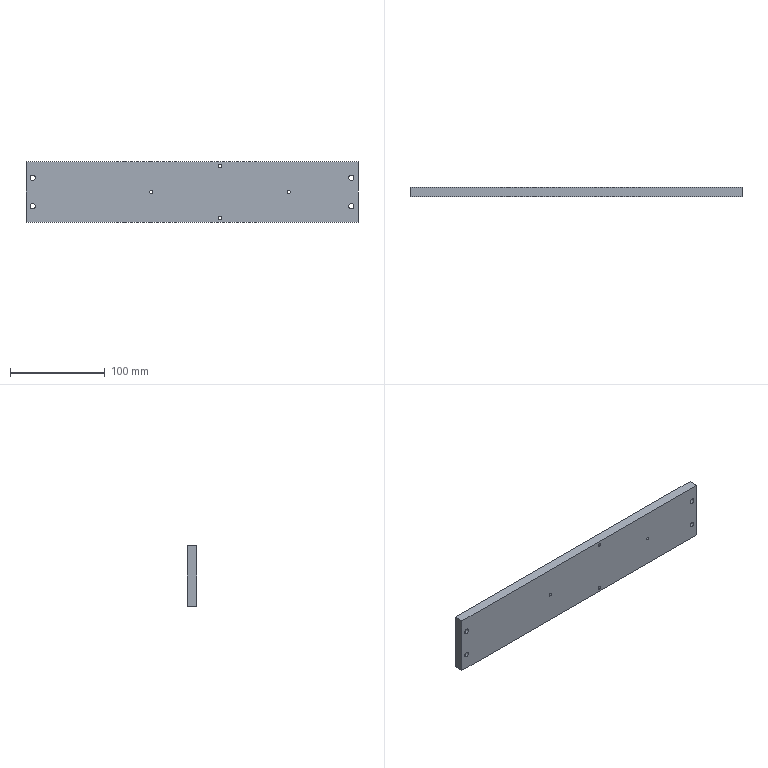Part | STEP file | PN_0015 spacer block | 1 solid | 34 faces | box 350 x 10 x 64 mm | volume 221459 mm3 | cylinder 24 | plane 10 | commonest cylinder face diameters 3.3 x8 5.5 x8 10 x8